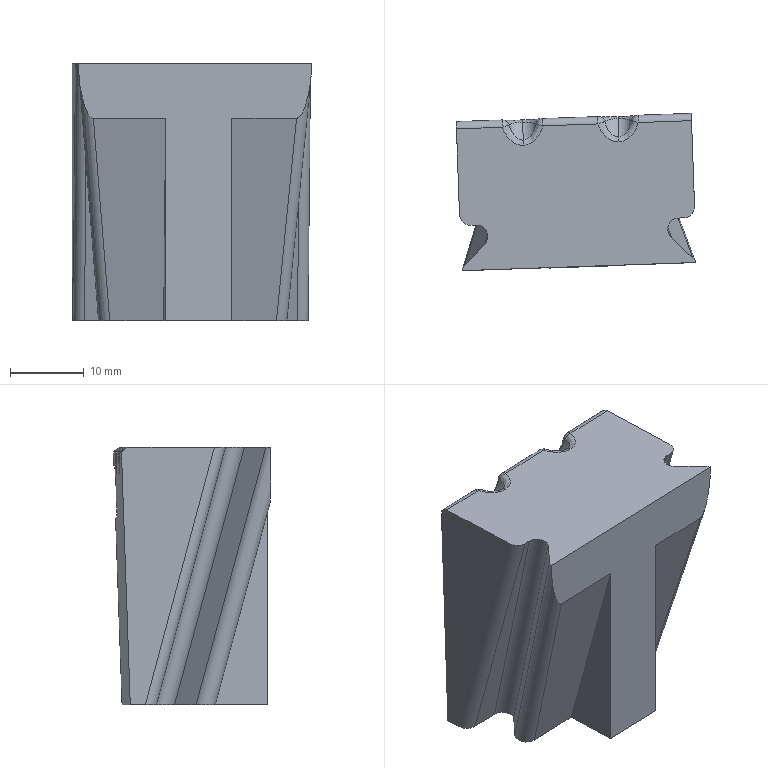Part | NX | features DIE-73 2 | 1 solid | 44 faces | box 32.592 x 21.404 x 35 mm | volume 17676 mm3 | plane 17 | spline 14 | cylinder 9 | sphere 4 | commonest cylinder face diameters 3 x6 2 x3